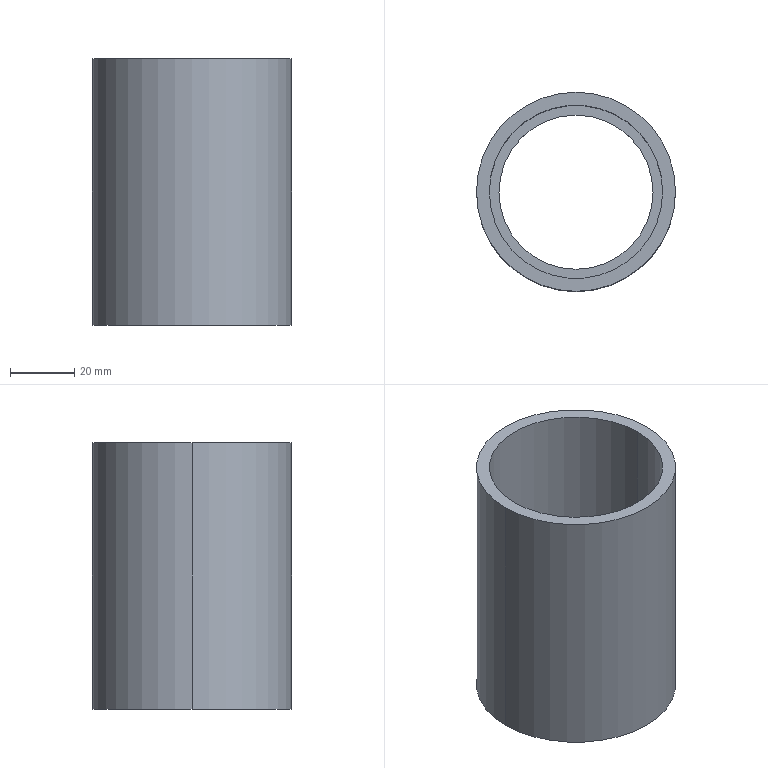Part | STEP file | Tube locking nut | 1 solid | 9 faces | box 62 x 62 x 83 mm | volume 61936 mm3 | cylinder 6 | plane 3 | commonest cylinder face diameters 48 x2 54 x2 62 x2
STEP:
#1=CARTESIAN_POINT('',(0.,0.,0.));
#2=DIRECTION('',(0.,0.,1.));
#3=DIRECTION('',(1.,0.,0.));
#4=AXIS2_PLACEMENT_3D('',#1,#2,#3);
#5=CARTESIAN_POINT('',(-27.,0.,83.));
#6=VERTEX_POINT('',#5);
#7=CARTESIAN_POINT('',(-27.,0.,3.));
#8=VERTEX_POINT('',#7);
#9=CARTESIAN_POINT('',(-27.,0.,83.));
#10=DIRECTION('',(0.,0.,-1.));
#11=VECTOR('',#10,1.);
#12=LINE('',#9,#11);
#13=CARTESIAN_POINT('',(0.,0.,83.));
#14=DIRECTION('',(0.,0.,-1.));
#15=DIRECTION('',(-1.,0.,0.));
#16=AXIS2_PLACEMENT_3D('',#13,#14,#15);
#17=CYLINDRICAL_SURFACE('',#16,27.);
#18=CARTESIAN_POINT('',(6.283,0.));
#19=DIRECTION('',(0.,1.));
#20=VECTOR('',#19,1.);
#21=LINE('',#18,#20);
#22=(GEOMETRIC_REPRESENTATION_CONTEXT(2)PARAMETRIC_REPRESENTATION_CONTEXT()REPRESENTATION_CONTEXT('',''));
#23=DEFINITIONAL_REPRESENTATION('',(#21),#22);
#24=PCURVE('',#17,#23);
#25=CARTESIAN_POINT('',(0.,0.,83.));
#26=DIRECTION('',(0.,0.,-1.));
#27=DIRECTION('',(-1.,0.,0.));
#28=AXIS2_PLACEMENT_3D('',#25,#26,#27);
#29=CYLINDRICAL_SURFACE('',#28,27.);
#30=CARTESIAN_POINT('',(0.,0.));
#31=DIRECTION('',(0.,1.));
#32=VECTOR('',#31,1.);
#33=LINE('',#30,#32);
#34=(GEOMETRIC_REPRESENTATION_CONTEXT(2)PARAMETRIC_REPRESENTATION_CONTEXT()REPRESENTATION_CONTEXT('',''));
#35=DEFINITIONAL_REPRESENTATION('',(#33),#34);
#36=PCURVE('',#29,#35);
#37=SURFACE_CURVE('',#12,(#24,#36),.PCURVE_S1.);
#38=EDGE_CURVE('',#6,#8,#37,.T.);
#39=ORIENTED_EDGE('',*,*,#38,.T.);
#40=CARTESIAN_POINT('',(27.,0.,3.));
#41=VERTEX_POINT('',#40);
#42=CARTESIAN_POINT('',(0.,0.,3.));
#43=DIRECTION('',(0.,0.,1.));
#44=DIRECTION('',(1.,0.,0.));
#45=AXIS2_PLACEMENT_3D('',#42,#43,#44);
#46=CIRCLE('',#45,27.);
#47=CARTESIAN_POINT('',(9.425,80.));
#48=DIRECTION('',(-1.,0.));
#49=VECTOR('',#48,1.);
#50=LINE('',#47,#49);
#51=(GEOMETRIC_REPRESENTATION_CONTEXT(2)PARAMETRIC_REPRESENTATION_CONTEXT()REPRESENTATION_CONTEXT('',''));
#52=DEFINITIONAL_REPRESENTATION('',(#50),#51);
#53=PCURVE('',#17,#52);
#54=CARTESIAN_POINT('',(0.,0.,3.));
#55=DIRECTION('',(0.,0.,1.));
#56=DIRECTION('',(1.,0.,0.));
#57=AXIS2_PLACEMENT_3D('',#54,#55,#56);
#58=PLANE('',#57);
#59=CARTESIAN_POINT('',(0.,0.));
#60=DIRECTION('',(1.,0.));
#61=AXIS2_PLACEMENT_2D('',#59,#60);
#62=CIRCLE('',#61,27.);
#63=(GEOMETRIC_REPRESENTATION_CONTEXT(2)PARAMETRIC_REPRESENTATION_CONTEXT()REPRESENTATION_CONTEXT('',''));
#64=DEFINITIONAL_REPRESENTATION('',(#62),#63);
#65=PCURVE('',#58,#64);
#66=SURFACE_CURVE('',#46,(#53,#65),.PCURVE_S1.);
#67=EDGE_CURVE('',#8,#41,#66,.T.);
#68=ORIENTED_EDGE('',*,*,#67,.T.);
#69=CARTESIAN_POINT('',(27.,0.,83.));
#70=VERTEX_POINT('',#69);
#71=CARTESIAN_POINT('',(27.,0.,83.));
#72=DIRECTION('',(0.,0.,-1.));
#73=VECTOR('',#72,1.);
#74=LINE('',#71,#73);
#75=CARTESIAN_POINT('',(3.142,0.));
#76=DIRECTION('',(0.,1.));
#77=VECTOR('',#76,1.);
#78=LINE('',#75,#77);
#79=(GEOMETRIC_REPRESENTATION_CONTEXT(2)PARAMETRIC_REPRESENTATION_CONTEXT()REPRESENTATION_CONTEXT('',''));
#80=DEFINITIONAL_REPRESENTATION('',(#78),#79);
#81=PCURVE('',#17,#80);
#82=CARTESIAN_POINT('',(3.142,0.));
#83=DIRECTION('',(0.,1.));
#84=VECTOR('',#83,1.);
#85=LINE('',#82,#84);
#86=(GEOMETRIC_REPRESENTATION_CONTEXT(2)PARAMETRIC_REPRESENTATION_CONTEXT()REPRESENTATION_CONTEXT('',''));
#87=DEFINITIONAL_REPRESENTATION('',(#85),#86);
#88=PCURVE('',#29,#87);
#89=SURFACE_CURVE('',#74,(#81,#88),.PCURVE_S1.);
#90=EDGE_CURVE('',#70,#41,#89,.T.);
#91=ORIENTED_EDGE('',*,*,#90,.F.);
#92=CARTESIAN_POINT('',(0.,0.,83.));
#93=DIRECTION('',(0.,0.,1.));
#94=DIRECTION('',(1.,0.,0.));
#95=AXIS2_PLACEMENT_3D('',#92,#93,#94);
#96=CIRCLE('',#95,27.);
#97=CARTESIAN_POINT('',(9.425,0.));
#98=DIRECTION('',(-1.,0.));
#99=VECTOR('',#98,1.);
#100=LINE('',#97,#99);
#101=(GEOMETRIC_REPRESENTATION_CONTEXT(2)PARAMETRIC_REPRESENTATION_CONTEXT()REPRESENTATION_CONTEXT('',''));
#102=DEFINITIONAL_REPRESENTATION('',(#100),#101);
#103=PCURVE('',#17,#102);
#104=CARTESIAN_POINT('',(0.,0.,83.));
#105=DIRECTION('',(0.,0.,1.));
#106=DIRECTION('',(1.,0.,0.));
#107=AXIS2_PLACEMENT_3D('',#104,#105,#106);
#108=PLANE('',#107);
#109=CARTESIAN_POINT('',(0.,0.));
#110=DIRECTION('',(1.,0.));
#111=AXIS2_PLACEMENT_2D('',#109,#110);
#112=CIRCLE('',#111,27.);
#113=(GEOMETRIC_REPRESENTATION_CONTEXT(2)PARAMETRIC_REPRESENTATION_CONTEXT()REPRESENTATION_CONTEXT('',''));
#114=DEFINITIONAL_REPRESENTATION('',(#112),#113);
#115=PCURVE('',#108,#114);
#116=SURFACE_CURVE('',#96,(#103,#115),.PCURVE_S1.);
#117=EDGE_CURVE('',#6,#70,#116,.T.);
#118=ORIENTED_EDGE('',*,*,#117,.F.);
#119=EDGE_LOOP('',(#39,#68,#91,#118));
#120=FACE_BOUND('',#119,.F.);
#121=ADVANCED_FACE('',(#120),#17,.F.);
#122=CARTESIAN_POINT('',(-24.,0.,3.));
#123=VERTEX_POINT('',#122);
#124=CARTESIAN_POINT('',(-24.,0.,0.));
#125=VERTEX_POINT('',#124);
#126=CARTESIAN_POINT('',(-24.,0.,3.));
#127=DIRECTION('',(0.,0.,-1.));
#128=VECTOR('',#127,1.);
#129=LINE('',#126,#128);
#130=CARTESIAN_POINT('',(0.,0.,3.));
#131=DIRECTION('',(0.,0.,-1.));
#132=DIRECTION('',(-1.,0.,0.));
#133=AXIS2_PLACEMENT_3D('',#130,#131,#132);
#134=CYLINDRICAL_SURFACE('',#133,24.);
#135=CARTESIAN_POINT('',(6.283,0.));
#136=DIRECTION('',(0.,1.));
#137=VECTOR('',#136,1.);
#138=LINE('',#135,#137);
#139=(GEOMETRIC_REPRESENTATION_CONTEXT(2)PARAMETRIC_REPRESENTATION_CONTEXT()REPRESENTATION_CONTEXT('',''));
#140=DEFINITIONAL_REPRESENTATION('',(#138),#139);
#141=PCURVE('',#134,#140);
#142=CARTESIAN_POINT('',(0.,0.,3.));
#143=DIRECTION('',(0.,0.,-1.));
#144=DIRECTION('',(-1.,0.,0.));
#145=AXIS2_PLACEMENT_3D('',#142,#143,#144);
#146=CYLINDRICAL_SURFACE('',#145,24.);
#147=CARTESIAN_POINT('',(0.,0.));
#148=DIRECTION('',(0.,1.));
#149=VECTOR('',#148,1.);
#150=LINE('',#147,#149);
#151=(GEOMETRIC_REPRESENTATION_CONTEXT(2)PARAMETRIC_REPRESENTATION_CONTEXT()REPRESENTATION_CONTEXT('',''));
#152=DEFINITIONAL_REPRESENTATION('',(#150),#151);
#153=PCURVE('',#146,#152);
#154=SURFACE_CURVE('',#129,(#141,#153),.PCURVE_S1.);
#155=EDGE_CURVE('',#123,#125,#154,.T.);
#156=ORIENTED_EDGE('',*,*,#155,.T.);
#157=CARTESIAN_POINT('',(24.,0.,0.));
#158=VERTEX_POINT('',#157);
#159=CARTESIAN_POINT('',(0.,0.,0.));
#160=DIRECTION('',(0.,0.,1.));
#161=DIRECTION('',(1.,0.,0.));
#162=AXIS2_PLACEMENT_3D('',#159,#160,#161);
#163=CIRCLE('',#162,24.);
#164=CARTESIAN_POINT('',(9.425,3.));
#165=DIRECTION('',(-1.,0.));
#166=VECTOR('',#165,1.);
#167=LINE('',#164,#166);
#168=(GEOMETRIC_REPRESENTATION_CONTEXT(2)PARAMETRIC_REPRESENTATION_CONTEXT()REPRESENTATION_CONTEXT('',''));
#169=DEFINITIONAL_REPRESENTATION('',(#167),#168);
#170=PCURVE('',#134,#169);
#171=CARTESIAN_POINT('',(0.,0.,0.));
#172=DIRECTION('',(0.,0.,1.));
#173=DIRECTION('',(1.,0.,0.));
#174=AXIS2_PLACEMENT_3D('',#171,#172,#173);
#175=PLANE('',#174);
#176=CARTESIAN_POINT('',(0.,0.));
#177=DIRECTION('',(1.,0.));
#178=AXIS2_PLACEMENT_2D('',#176,#177);
#179=CIRCLE('',#178,24.);
#180=(GEOMETRIC_REPRESENTATION_CONTEXT(2)PARAMETRIC_REPRESENTATION_CONTEXT()REPRESENTATION_CONTEXT('',''));
#181=DEFINITIONAL_REPRESENTATION('',(#179),#180);
#182=PCURVE('',#175,#181);
#183=SURFACE_CURVE('',#163,(#170,#182),.PCURVE_S1.);
#184=EDGE_CURVE('',#125,#158,#183,.T.);
#185=ORIENTED_EDGE('',*,*,#184,.T.);
#186=CARTESIAN_POINT('',(24.,0.,3.));
#187=VERTEX_POINT('',#186);
#188=CARTESIAN_POINT('',(24.,0.,3.));
#189=DIRECTION('',(0.,0.,-1.));
#190=VECTOR('',#189,1.);
#191=LINE('',#188,#190);
#192=CARTESIAN_POINT('',(3.142,0.));
#193=DIRECTION('',(0.,1.));
#194=VECTOR('',#193,1.);
#195=LINE('',#192,#194);
#196=(GEOMETRIC_REPRESENTATION_CONTEXT(2)PARAMETRIC_REPRESENTATION_CONTEXT()REPRESENTATION_CONTEXT('',''));
#197=DEFINITIONAL_REPRESENTATION('',(#195),#196);
#198=PCURVE('',#134,#197);
#199=CARTESIAN_POINT('',(3.142,0.));
#200=DIRECTION('',(0.,1.));
#201=VECTOR('',#200,1.);
#202=LINE('',#199,#201);
#203=(GEOMETRIC_REPRESENTATION_CONTEXT(2)PARAMETRIC_REPRESENTATION_CONTEXT()REPRESENTATION_CONTEXT('',''));
#204=DEFINITIONAL_REPRESENTATION('',(#202),#203);
#205=PCURVE('',#146,#204);
#206=SURFACE_CURVE('',#191,(#198,#205),.PCURVE_S1.);
#207=EDGE_CURVE('',#187,#158,#206,.T.);
#208=ORIENTED_EDGE('',*,*,#207,.F.);
#209=CARTESIAN_POINT('',(0.,0.,3.));
#210=DIRECTION('',(0.,0.,1.));
#211=DIRECTION('',(1.,0.,0.));
#212=AXIS2_PLACEMENT_3D('',#209,#210,#211);
#213=CIRCLE('',#212,24.);
#214=CARTESIAN_POINT('',(9.425,0.));
#215=DIRECTION('',(-1.,0.));
#216=VECTOR('',#215,1.);
#217=LINE('',#214,#216);
#218=(GEOMETRIC_REPRESENTATION_CONTEXT(2)PARAMETRIC_REPRESENTATION_CONTEXT()REPRESENTATION_CONTEXT('',''));
#219=DEFINITIONAL_REPRESENTATION('',(#217),#218);
#220=PCURVE('',#134,#219);
#221=CARTESIAN_POINT('',(0.,0.));
#222=DIRECTION('',(1.,0.));
#223=AXIS2_PLACEMENT_2D('',#221,#222);
#224=CIRCLE('',#223,24.);
#225=(GEOMETRIC_REPRESENTATION_CONTEXT(2)PARAMETRIC_REPRESENTATION_CONTEXT()REPRESENTATION_CONTEXT('',''));
#226=DEFINITIONAL_REPRESENTATION('',(#224),#225);
#227=PCURVE('',#58,#226);
#228=SURFACE_CURVE('',#213,(#220,#227),.PCURVE_S1.);
#229=EDGE_CURVE('',#123,#187,#228,.T.);
#230=ORIENTED_EDGE('',*,*,#229,.F.);
#231=EDGE_LOOP('',(#156,#185,#208,#230));
#232=FACE_BOUND('',#231,.F.);
#233=ADVANCED_FACE('',(#232),#134,.F.);
#234=CARTESIAN_POINT('',(31.,0.,83.));
#235=VERTEX_POINT('',#234);
#236=CARTESIAN_POINT('',(-31.,0.,83.));
#237=VERTEX_POINT('',#236);
#238=CARTESIAN_POINT('',(0.,0.,83.));
#239=DIRECTION('',(0.,0.,1.));
#240=DIRECTION('',(1.,0.,0.));
#241=AXIS2_PLACEMENT_3D('',#238,#239,#240);
#242=CIRCLE('',#241,31.);
#243=CARTESIAN_POINT('',(0.,0.,3.));
#244=DIRECTION('',(0.,0.,-1.));
#245=DIRECTION('',(-1.,0.,0.));
#246=AXIS2_PLACEMENT_3D('',#243,#244,#245);
#247=CYLINDRICAL_SURFACE('',#246,31.);
#248=CARTESIAN_POINT('',(3.142,-80.));
#249=DIRECTION('',(-1.,0.));
#250=VECTOR('',#249,1.);
#251=LINE('',#248,#250);
#252=(GEOMETRIC_REPRESENTATION_CONTEXT(2)PARAMETRIC_REPRESENTATION_CONTEXT()REPRESENTATION_CONTEXT('',''));
#253=DEFINITIONAL_REPRESENTATION('',(#251),#252);
#254=PCURVE('',#247,#253);
#255=CARTESIAN_POINT('',(0.,0.));
#256=DIRECTION('',(1.,0.));
#257=AXIS2_PLACEMENT_2D('',#255,#256);
#258=CIRCLE('',#257,31.);
#259=(GEOMETRIC_REPRESENTATION_CONTEXT(2)PARAMETRIC_REPRESENTATION_CONTEXT()REPRESENTATION_CONTEXT('',''));
#260=DEFINITIONAL_REPRESENTATION('',(#258),#259);
#261=PCURVE('',#108,#260);
#262=SURFACE_CURVE('',#242,(#254,#261),.PCURVE_S1.);
#263=EDGE_CURVE('',#235,#237,#262,.T.);
#264=ORIENTED_EDGE('',*,*,#263,.F.);
#265=CARTESIAN_POINT('',(31.,0.,0.));
#266=VERTEX_POINT('',#265);
#267=CARTESIAN_POINT('',(31.,0.,3.));
#268=DIRECTION('',(0.,0.,-1.));
#269=VECTOR('',#268,1.);
#270=LINE('',#267,#269);
#271=CARTESIAN_POINT('',(3.142,0.));
#272=DIRECTION('',(0.,1.));
#273=VECTOR('',#272,1.);
#274=LINE('',#271,#273);
#275=(GEOMETRIC_REPRESENTATION_CONTEXT(2)PARAMETRIC_REPRESENTATION_CONTEXT()REPRESENTATION_CONTEXT('',''));
#276=DEFINITIONAL_REPRESENTATION('',(#274),#275);
#277=PCURVE('',#247,#276);
#278=CARTESIAN_POINT('',(0.,0.,3.));
#279=DIRECTION('',(0.,0.,-1.));
#280=DIRECTION('',(-1.,0.,0.));
#281=AXIS2_PLACEMENT_3D('',#278,#279,#280);
#282=CYLINDRICAL_SURFACE('',#281,31.);
#283=CARTESIAN_POINT('',(3.142,0.));
#284=DIRECTION('',(0.,1.));
#285=VECTOR('',#284,1.);
#286=LINE('',#283,#285);
#287=(GEOMETRIC_REPRESENTATION_CONTEXT(2)PARAMETRIC_REPRESENTATION_CONTEXT()REPRESENTATION_CONTEXT('',''));
#288=DEFINITIONAL_REPRESENTATION('',(#286),#287);
#289=PCURVE('',#282,#288);
#290=SURFACE_CURVE('',#270,(#277,#289),.PCURVE_S1.);
#291=EDGE_CURVE('',#235,#266,#290,.T.);
#292=ORIENTED_EDGE('',*,*,#291,.T.);
#293=CARTESIAN_POINT('',(-31.,0.,0.));
#294=VERTEX_POINT('',#293);
#295=CARTESIAN_POINT('',(0.,0.,0.));
#296=DIRECTION('',(0.,0.,1.));
#297=DIRECTION('',(1.,0.,0.));
#298=AXIS2_PLACEMENT_3D('',#295,#296,#297);
#299=CIRCLE('',#298,31.);
#300=CARTESIAN_POINT('',(3.142,3.));
#301=DIRECTION('',(-1.,0.));
#302=VECTOR('',#301,1.);
#303=LINE('',#300,#302);
#304=(GEOMETRIC_REPRESENTATION_CONTEXT(2)PARAMETRIC_REPRESENTATION_CONTEXT()REPRESENTATION_CONTEXT('',''));
#305=DEFINITIONAL_REPRESENTATION('',(#303),#304);
#306=PCURVE('',#247,#305);
#307=CARTESIAN_POINT('',(0.,0.));
#308=DIRECTION('',(1.,0.));
#309=AXIS2_PLACEMENT_2D('',#307,#308);
#310=CIRCLE('',#309,31.);
#311=(GEOMETRIC_REPRESENTATION_CONTEXT(2)PARAMETRIC_REPRESENTATION_CONTEXT()REPRESENTATION_CONTEXT('',''));
#312=DEFINITIONAL_REPRESENTATION('',(#310),#311);
#313=PCURVE('',#175,#312);
#314=SURFACE_CURVE('',#299,(#306,#313),.PCURVE_S1.);
#315=EDGE_CURVE('',#266,#294,#314,.T.);
#316=ORIENTED_EDGE('',*,*,#315,.T.);
#317=CARTESIAN_POINT('',(-31.,0.,3.));
#318=DIRECTION('',(0.,0.,-1.));
#319=VECTOR('',#318,1.);
#320=LINE('',#317,#319);
#321=CARTESIAN_POINT('',(0.,0.));
#322=DIRECTION('',(0.,1.));
#323=VECTOR('',#322,1.);
#324=LINE('',#321,#323);
#325=(GEOMETRIC_REPRESENTATION_CONTEXT(2)PARAMETRIC_REPRESENTATION_CONTEXT()REPRESENTATION_CONTEXT('',''));
#326=DEFINITIONAL_REPRESENTATION('',(#324),#325);
#327=PCURVE('',#247,#326);
#328=CARTESIAN_POINT('',(6.283,0.));
#329=DIRECTION('',(0.,1.));
#330=VECTOR('',#329,1.);
#331=LINE('',#328,#330);
#332=(GEOMETRIC_REPRESENTATION_CONTEXT(2)PARAMETRIC_REPRESENTATION_CONTEXT()REPRESENTATION_CONTEXT('',''));
#333=DEFINITIONAL_REPRESENTATION('',(#331),#332);
#334=PCURVE('',#282,#333);
#335=SURFACE_CURVE('',#320,(#327,#334),.PCURVE_S1.);
#336=EDGE_CURVE('',#237,#294,#335,.T.);
#337=ORIENTED_EDGE('',*,*,#336,.F.);
#338=EDGE_LOOP('',(#264,#292,#316,#337));
#339=FACE_BOUND('',#338,.T.);
#340=ADVANCED_FACE('',(#339),#247,.T.);
#341=ORIENTED_EDGE('',*,*,#229,.F.);
#342=CARTESIAN_POINT('',(0.,0.,3.));
#343=DIRECTION('',(0.,0.,1.));
#344=DIRECTION('',(1.,0.,0.));
#345=AXIS2_PLACEMENT_3D('',#342,#343,#344);
#346=CIRCLE('',#345,24.);
#347=CARTESIAN_POINT('',(0.,0.));
#348=DIRECTION('',(1.,0.));
#349=AXIS2_PLACEMENT_2D('',#347,#348);
#350=CIRCLE('',#349,24.);
#351=(GEOMETRIC_REPRESENTATION_CONTEXT(2)PARAMETRIC_REPRESENTATION_CONTEXT()REPRESENTATION_CONTEXT('',''));
#352=DEFINITIONAL_REPRESENTATION('',(#350),#351);
#353=PCURVE('',#58,#352);
#354=CARTESIAN_POINT('',(3.142,0.));
#355=DIRECTION('',(-1.,0.));
#356=VECTOR('',#355,1.);
#357=LINE('',#354,#356);
#358=(GEOMETRIC_REPRESENTATION_CONTEXT(2)PARAMETRIC_REPRESENTATION_CONTEXT()REPRESENTATION_CONTEXT('',''));
#359=DEFINITIONAL_REPRESENTATION('',(#357),#358);
#360=PCURVE('',#146,#359);
#361=SURFACE_CURVE('',#346,(#353,#360),.PCURVE_S1.);
#362=EDGE_CURVE('',#187,#123,#361,.T.);
#363=ORIENTED_EDGE('',*,*,#362,.F.);
#364=EDGE_LOOP('',(#341,#363));
#365=FACE_BOUND('',#364,.T.);
#366=ORIENTED_EDGE('',*,*,#67,.T.);
#367=CARTESIAN_POINT('',(0.,0.,3.));
#368=DIRECTION('',(0.,0.,1.));
#369=DIRECTION('',(1.,0.,0.));
#370=AXIS2_PLACEMENT_3D('',#367,#368,#369);
#371=CIRCLE('',#370,27.);
#372=CARTESIAN_POINT('',(0.,0.));
#373=DIRECTION('',(1.,0.));
#374=AXIS2_PLACEMENT_2D('',#372,#373);
#375=CIRCLE('',#374,27.);
#376=(GEOMETRIC_REPRESENTATION_CONTEXT(2)PARAMETRIC_REPRESENTATION_CONTEXT()REPRESENTATION_CONTEXT('',''));
#377=DEFINITIONAL_REPRESENTATION('',(#375),#376);
#378=PCURVE('',#58,#377);
#379=CARTESIAN_POINT('',(3.142,80.));
#380=DIRECTION('',(-1.,0.));
#381=VECTOR('',#380,1.);
#382=LINE('',#379,#381);
#383=(GEOMETRIC_REPRESENTATION_CONTEXT(2)PARAMETRIC_REPRESENTATION_CONTEXT()REPRESENTATION_CONTEXT('',''));
#384=DEFINITIONAL_REPRESENTATION('',(#382),#383);
#385=PCURVE('',#29,#384);
#386=SURFACE_CURVE('',#371,(#378,#385),.PCURVE_S1.);
#387=EDGE_CURVE('',#41,#8,#386,.T.);
#388=ORIENTED_EDGE('',*,*,#387,.T.);
#389=EDGE_LOOP('',(#366,#388));
#390=FACE_BOUND('',#389,.T.);
#391=ADVANCED_FACE('',(#365,#390),#58,.T.);
#392=CARTESIAN_POINT('',(0.,0.,0.));
#393=DIRECTION('',(0.,0.,1.));
#394=DIRECTION('',(1.,0.,0.));
#395=AXIS2_PLACEMENT_3D('',#392,#393,#394);
#396=CIRCLE('',#395,31.);
#397=CARTESIAN_POINT('',(0.,0.));
#398=DIRECTION('',(1.,0.));
#399=AXIS2_PLACEMENT_2D('',#397,#398);
#400=CIRCLE('',#399,31.);
#401=(GEOMETRIC_REPRESENTATION_CONTEXT(2)PARAMETRIC_REPRESENTATION_CONTEXT()REPRESENTATION_CONTEXT('',''));
#402=DEFINITIONAL_REPRESENTATION('',(#400),#401);
#403=PCURVE('',#175,#402);
#404=CARTESIAN_POINT('',(9.425,3.));
#405=DIRECTION('',(-1.,0.));
#406=VECTOR('',#405,1.);
#407=LINE('',#404,#406);
#408=(GEOMETRIC_REPRESENTATION_CONTEXT(2)PARAMETRIC_REPRESENTATION_CONTEXT()REPRESENTATION_CONTEXT('',''));
#409=DEFINITIONAL_REPRESENTATION('',(#407),#408);
#410=PCURVE('',#282,#409);
#411=SURFACE_CURVE('',#396,(#403,#410),.PCURVE_S1.);
#412=EDGE_CURVE('',#294,#266,#411,.T.);
#413=ORIENTED_EDGE('',*,*,#412,.F.);
#414=ORIENTED_EDGE('',*,*,#315,.F.);
#415=EDGE_LOOP('',(#413,#414));
#416=FACE_BOUND('',#415,.T.);
#417=ORIENTED_EDGE('',*,*,#184,.T.);
#418=CARTESIAN_POINT('',(0.,0.,0.));
#419=DIRECTION('',(0.,0.,1.));
#420=DIRECTION('',(1.,0.,0.));
#421=AXIS2_PLACEMENT_3D('',#418,#419,#420);
#422=CIRCLE('',#421,24.);
#423=CARTESIAN_POINT('',(0.,0.));
#424=DIRECTION('',(1.,0.));
#425=AXIS2_PLACEMENT_2D('',#423,#424);
#426=CIRCLE('',#425,24.);
#427=(GEOMETRIC_REPRESENTATION_CONTEXT(2)PARAMETRIC_REPRESENTATION_CONTEXT()REPRESENTATION_CONTEXT('',''));
#428=DEFINITIONAL_REPRESENTATION('',(#426),#427);
#429=PCURVE('',#175,#428);
#430=CARTESIAN_POINT('',(3.142,3.));
#431=DIRECTION('',(-1.,0.));
#432=VECTOR('',#431,1.);
#433=LINE('',#430,#432);
#434=(GEOMETRIC_REPRESENTATION_CONTEXT(2)PARAMETRIC_REPRESENTATION_CONTEXT()REPRESENTATION_CONTEXT('',''));
#435=DEFINITIONAL_REPRESENTATION('',(#433),#434);
#436=PCURVE('',#146,#435);
#437=SURFACE_CURVE('',#422,(#429,#436),.PCURVE_S1.);
#438=EDGE_CURVE('',#158,#125,#437,.T.);
#439=ORIENTED_EDGE('',*,*,#438,.T.);
#440=EDGE_LOOP('',(#417,#439));
#441=FACE_BOUND('',#440,.T.);
#442=ADVANCED_FACE('',(#416,#441),#175,.F.);
#443=ORIENTED_EDGE('',*,*,#291,.F.);
#444=CARTESIAN_POINT('',(0.,0.,83.));
#445=DIRECTION('',(0.,0.,1.));
#446=DIRECTION('',(1.,0.,0.));
#447=AXIS2_PLACEMENT_3D('',#444,#445,#446);
#448=CIRCLE('',#447,31.);
#449=CARTESIAN_POINT('',(9.425,-80.));
#450=DIRECTION('',(-1.,0.));
#451=VECTOR('',#450,1.);
#452=LINE('',#449,#451);
#453=(GEOMETRIC_REPRESENTATION_CONTEXT(2)PARAMETRIC_REPRESENTATION_CONTEXT()REPRESENTATION_CONTEXT('',''));
#454=DEFINITIONAL_REPRESENTATION('',(#452),#453);
#455=PCURVE('',#282,#454);
#456=CARTESIAN_POINT('',(0.,0.));
#457=DIRECTION('',(1.,0.));
#458=AXIS2_PLACEMENT_2D('',#456,#457);
#459=CIRCLE('',#458,31.);
#460=(GEOMETRIC_REPRESENTATION_CONTEXT(2)PARAMETRIC_REPRESENTATION_CONTEXT()REPRESENTATION_CONTEXT('',''));
#461=DEFINITIONAL_REPRESENTATION('',(#459),#460);
#462=PCURVE('',#108,#461);
#463=SURFACE_CURVE('',#448,(#455,#462),.PCURVE_S1.);
#464=EDGE_CURVE('',#237,#235,#463,.T.);
#465=ORIENTED_EDGE('',*,*,#464,.F.);
#466=ORIENTED_EDGE('',*,*,#336,.T.);
#467=ORIENTED_EDGE('',*,*,#412,.T.);
#468=EDGE_LOOP('',(#443,#465,#466,#467));
#469=FACE_BOUND('',#468,.T.);
#470=ADVANCED_FACE('',(#469),#282,.T.);
#471=ORIENTED_EDGE('',*,*,#438,.T.);
#472=ORIENTED_EDGE('',*,*,#155,.F.);
#473=ORIENTED_EDGE('',*,*,#362,.F.);
#474=ORIENTED_EDGE('',*,*,#207,.T.);
#475=EDGE_LOOP('',(#471,#472,#473,#474));
#476=FACE_BOUND('',#475,.F.);
#477=ADVANCED_FACE('',(#476),#146,.F.);
#478=ORIENTED_EDGE('',*,*,#464,.T.);
#479=ORIENTED_EDGE('',*,*,#263,.T.);
#480=EDGE_LOOP('',(#478,#479));
#481=FACE_BOUND('',#480,.T.);
#482=ORIENTED_EDGE('',*,*,#117,.F.);
#483=CARTESIAN_POINT('',(0.,0.,83.));
#484=DIRECTION('',(0.,0.,1.));
#485=DIRECTION('',(1.,0.,0.));
#486=AXIS2_PLACEMENT_3D('',#483,#484,#485);
#487=CIRCLE('',#486,27.);
#488=CARTESIAN_POINT('',(0.,0.));
#489=DIRECTION('',(1.,0.));
#490=AXIS2_PLACEMENT_2D('',#488,#489);
#491=CIRCLE('',#490,27.);
#492=(GEOMETRIC_REPRESENTATION_CONTEXT(2)PARAMETRIC_REPRESENTATION_CONTEXT()REPRESENTATION_CONTEXT('',''));
#493=DEFINITIONAL_REPRESENTATION('',(#491),#492);
#494=PCURVE('',#108,#493);
#495=CARTESIAN_POINT('',(3.142,0.));
#496=DIRECTION('',(-1.,0.));
#497=VECTOR('',#496,1.);
#498=LINE('',#495,#497);
#499=(GEOMETRIC_REPRESENTATION_CONTEXT(2)PARAMETRIC_REPRESENTATION_CONTEXT()REPRESENTATION_CONTEXT('',''));
#500=DEFINITIONAL_REPRESENTATION('',(#498),#499);
#501=PCURVE('',#29,#500);
#502=SURFACE_CURVE('',#487,(#494,#501),.PCURVE_S1.);
#503=EDGE_CURVE('',#70,#6,#502,.T.);
#504=ORIENTED_EDGE('',*,*,#503,.F.);
#505=EDGE_LOOP('',(#482,#504));
#506=FACE_BOUND('',#505,.T.);
#507=ADVANCED_FACE('',(#481,#506),#108,.T.);
#508=ORIENTED_EDGE('',*,*,#387,.T.);
#509=ORIENTED_EDGE('',*,*,#38,.F.);
#510=ORIENTED_EDGE('',*,*,#503,.F.);
#511=ORIENTED_EDGE('',*,*,#90,.T.);
#512=EDGE_LOOP('',(#508,#509,#510,#511));
#513=FACE_BOUND('',#512,.F.);
#514=ADVANCED_FACE('',(#513),#29,.F.);
#515=CLOSED_SHELL('',(#121,#233,#340,#391,#442,#470,#477,#507,#514));
#516=MANIFOLD_SOLID_BREP('',#515);
#517=(LENGTH_UNIT()NAMED_UNIT(*)SI_UNIT(.MILLI.,.METRE.));
#518=UNCERTAINTY_MEASURE_WITH_UNIT(LENGTH_MEASURE(0.0000001),#517,'','');
#519=(NAMED_UNIT(*)PLANE_ANGLE_UNIT()SI_UNIT($,.RADIAN.));
#520=(NAMED_UNIT(*)SI_UNIT($,.STERADIAN.)SOLID_ANGLE_UNIT());
#521=(GEOMETRIC_REPRESENTATION_CONTEXT(3)GLOBAL_UNCERTAINTY_ASSIGNED_CONTEXT((#518))GLOBAL_UNIT_ASSIGNED_CONTEXT((#517,#519,#520))REPRESENTATION_CONTEXT('',''));
#522=ADVANCED_BREP_SHAPE_REPRESENTATION('',(#4,#516),#521);